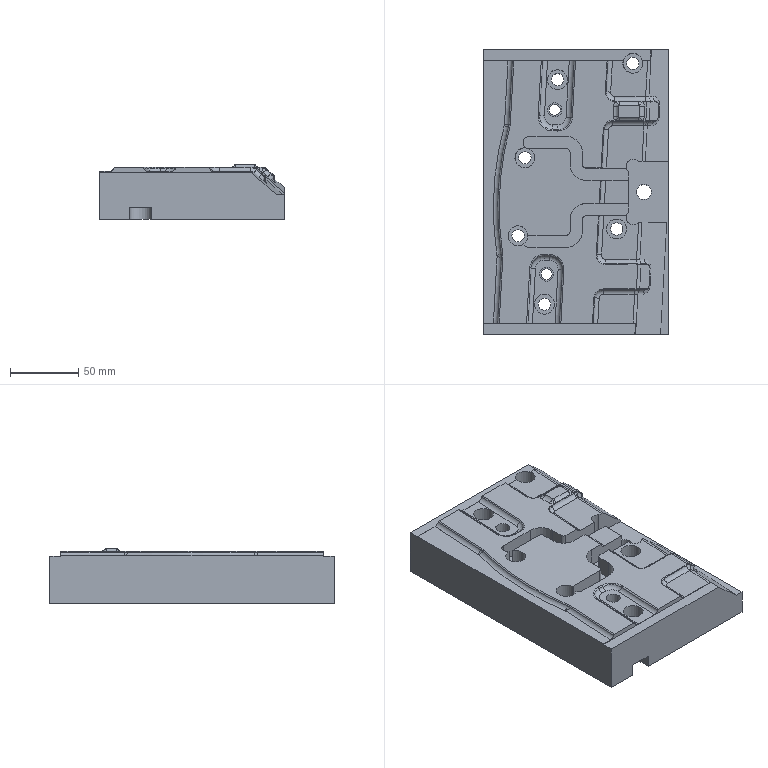Part | NX | features solid 2 | 1 solid | 213 faces | box 135 x 208 x 40 mm | volume 899790 mm3 | cylinder 93 | plane 62 | spline 36 | torus 22 | commonest cylinder face diameters 7 x27 1 x16 9 x10 2 x8 8 x7 14.5 x6